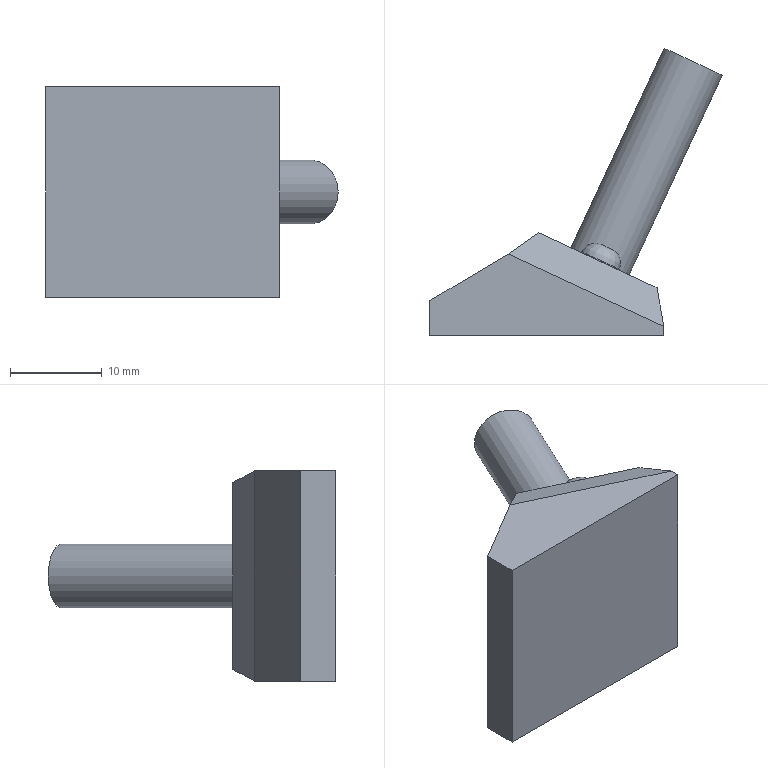Part | NX | 1 solid | 19 faces | box 31.865 x 31.333 x 22.9 mm | volume 5372 mm3 | plane 14 | cylinder 3 | spline 2 | commonest cylinder face diameters 4.5 x2 7 x1